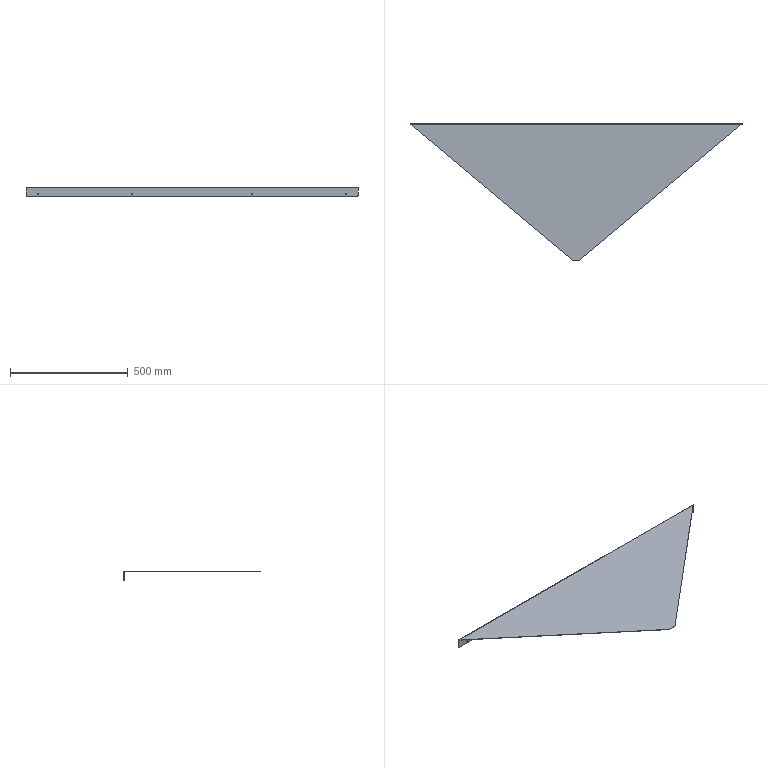Part | SolidWorks | features EdgeFlange 1, Fillet 1, FlatPattern 1, HoleWzd 1, SMBaseFlange 1, SheetMetal 1 | 1 solid | 24 faces | box 1412 x 580 x 40 mm | volume 567151 mm3 | cylinder 12 | plane 10 | spline 2 | commonest cylinder face diameters 4.5 x8 10 x2 0.2 x1 2.6 x1
STEP:
#1=CARTESIAN_POINT('',(50.,-1.2,-30.25));
#2=VERTEX_POINT('',#1);
#3=CARTESIAN_POINT('',(50.,-1.2,-25.75));
#4=VERTEX_POINT('',#3);
#5=CARTESIAN_POINT('',(50.,-1.2,-28.));
#6=DIRECTION('',(0.,1.,0.));
#7=DIRECTION('',(0.,0.,1.));
#8=AXIS2_PLACEMENT_3D('',#5,#6,#7);
#9=CIRCLE('',#8,2.25);
#10=EDGE_CURVE('',#2,#4,#9,.T.);
#11=ORIENTED_EDGE('',*,*,#10,.F.);
#12=CARTESIAN_POINT('',(50.,0.,-30.25));
#13=VERTEX_POINT('',#12);
#14=CARTESIAN_POINT('',(50.,0.,-30.25));
#15=DIRECTION('',(0.,1.,0.));
#16=VECTOR('',#15,1000.);
#17=LINE('',#14,#16);
#18=EDGE_CURVE('',#2,#13,#17,.T.);
#19=ORIENTED_EDGE('',*,*,#18,.T.);
#20=CARTESIAN_POINT('',(50.,0.,-25.75));
#21=VERTEX_POINT('',#20);
#22=CARTESIAN_POINT('',(50.,0.,-28.));
#23=DIRECTION('',(0.,1.,0.));
#24=DIRECTION('',(0.,0.,1.));
#25=AXIS2_PLACEMENT_3D('',#22,#23,#24);
#26=CIRCLE('',#25,2.25);
#27=EDGE_CURVE('',#13,#21,#26,.T.);
#28=ORIENTED_EDGE('',*,*,#27,.T.);
#29=CARTESIAN_POINT('',(50.,0.,-25.75));
#30=DIRECTION('',(0.,1.,0.));
#31=VECTOR('',#30,1000.);
#32=LINE('',#29,#31);
#33=EDGE_CURVE('',#4,#21,#32,.T.);
#34=ORIENTED_EDGE('',*,*,#33,.F.);
#35=EDGE_LOOP('',(#11,#19,#28,#34));
#36=FACE_OUTER_BOUND('',#35,.T.);
#37=CARTESIAN_POINT('',(50.,0.,-28.));
#38=DIRECTION('',(0.,1.,0.));
#39=DIRECTION('',(0.,0.,1.));
#40=AXIS2_PLACEMENT_3D('',#37,#38,#39);
#41=CYLINDRICAL_SURFACE('',#40,2.25);
#42=ADVANCED_FACE('',(#36),#41,.F.);
#43=CARTESIAN_POINT('',(1362.,-1.2,-30.25));
#44=VERTEX_POINT('',#43);
#45=CARTESIAN_POINT('',(1362.,-1.2,-25.75));
#46=VERTEX_POINT('',#45);
#47=CARTESIAN_POINT('',(1362.,-1.2,-28.));
#48=DIRECTION('',(0.,1.,0.));
#49=DIRECTION('',(0.,0.,1.));
#50=AXIS2_PLACEMENT_3D('',#47,#48,#49);
#51=CIRCLE('',#50,2.25);
#52=EDGE_CURVE('',#44,#46,#51,.T.);
#53=ORIENTED_EDGE('',*,*,#52,.F.);
#54=CARTESIAN_POINT('',(1362.,0.,-30.25));
#55=VERTEX_POINT('',#54);
#56=CARTESIAN_POINT('',(1362.,0.,-30.25));
#57=DIRECTION('',(0.,1.,0.));
#58=VECTOR('',#57,1000.);
#59=LINE('',#56,#58);
#60=EDGE_CURVE('',#44,#55,#59,.T.);
#61=ORIENTED_EDGE('',*,*,#60,.T.);
#62=CARTESIAN_POINT('',(1362.,0.,-25.75));
#63=VERTEX_POINT('',#62);
#64=CARTESIAN_POINT('',(1362.,0.,-28.));
#65=DIRECTION('',(0.,1.,0.));
#66=DIRECTION('',(0.,0.,1.));
#67=AXIS2_PLACEMENT_3D('',#64,#65,#66);
#68=CIRCLE('',#67,2.25);
#69=EDGE_CURVE('',#55,#63,#68,.T.);
#70=ORIENTED_EDGE('',*,*,#69,.T.);
#71=CARTESIAN_POINT('',(1362.,0.,-25.75));
#72=DIRECTION('',(0.,1.,0.));
#73=VECTOR('',#72,1000.);
#74=LINE('',#71,#73);
#75=EDGE_CURVE('',#46,#63,#74,.T.);
#76=ORIENTED_EDGE('',*,*,#75,.F.);
#77=EDGE_LOOP('',(#53,#61,#70,#76));
#78=FACE_OUTER_BOUND('',#77,.T.);
#79=CARTESIAN_POINT('',(1362.,0.,-28.));
#80=DIRECTION('',(0.,1.,0.));
#81=DIRECTION('',(0.,0.,1.));
#82=AXIS2_PLACEMENT_3D('',#79,#80,#81);
#83=CYLINDRICAL_SURFACE('',#82,2.25);
#84=ADVANCED_FACE('',(#78),#83,.F.);
#85=CARTESIAN_POINT('',(962.,-1.2,-30.25));
#86=VERTEX_POINT('',#85);
#87=CARTESIAN_POINT('',(962.,-1.2,-25.75));
#88=VERTEX_POINT('',#87);
#89=CARTESIAN_POINT('',(962.,-1.2,-28.));
#90=DIRECTION('',(0.,1.,0.));
#91=DIRECTION('',(0.,0.,1.));
#92=AXIS2_PLACEMENT_3D('',#89,#90,#91);
#93=CIRCLE('',#92,2.25);
#94=EDGE_CURVE('',#86,#88,#93,.T.);
#95=ORIENTED_EDGE('',*,*,#94,.F.);
#96=CARTESIAN_POINT('',(962.,0.,-30.25));
#97=VERTEX_POINT('',#96);
#98=CARTESIAN_POINT('',(962.,0.,-30.25));
#99=DIRECTION('',(0.,1.,0.));
#100=VECTOR('',#99,1000.);
#101=LINE('',#98,#100);
#102=EDGE_CURVE('',#86,#97,#101,.T.);
#103=ORIENTED_EDGE('',*,*,#102,.T.);
#104=CARTESIAN_POINT('',(962.,0.,-25.75));
#105=VERTEX_POINT('',#104);
#106=CARTESIAN_POINT('',(962.,0.,-28.));
#107=DIRECTION('',(0.,1.,0.));
#108=DIRECTION('',(0.,0.,1.));
#109=AXIS2_PLACEMENT_3D('',#106,#107,#108);
#110=CIRCLE('',#109,2.25);
#111=EDGE_CURVE('',#97,#105,#110,.T.);
#112=ORIENTED_EDGE('',*,*,#111,.T.);
#113=CARTESIAN_POINT('',(962.,0.,-25.75));
#114=DIRECTION('',(0.,1.,0.));
#115=VECTOR('',#114,1000.);
#116=LINE('',#113,#115);
#117=EDGE_CURVE('',#88,#105,#116,.T.);
#118=ORIENTED_EDGE('',*,*,#117,.F.);
#119=EDGE_LOOP('',(#95,#103,#112,#118));
#120=FACE_OUTER_BOUND('',#119,.T.);
#121=CARTESIAN_POINT('',(962.,0.,-28.));
#122=DIRECTION('',(0.,1.,0.));
#123=DIRECTION('',(0.,0.,1.));
#124=AXIS2_PLACEMENT_3D('',#121,#122,#123);
#125=CYLINDRICAL_SURFACE('',#124,2.25);
#126=ADVANCED_FACE('',(#120),#125,.F.);
#127=CARTESIAN_POINT('',(450.,-1.2,-30.25));
#128=VERTEX_POINT('',#127);
#129=CARTESIAN_POINT('',(450.,-1.2,-25.75));
#130=VERTEX_POINT('',#129);
#131=CARTESIAN_POINT('',(450.,-1.2,-28.));
#132=DIRECTION('',(0.,1.,0.));
#133=DIRECTION('',(0.,0.,1.));
#134=AXIS2_PLACEMENT_3D('',#131,#132,#133);
#135=CIRCLE('',#134,2.25);
#136=EDGE_CURVE('',#128,#130,#135,.T.);
#137=ORIENTED_EDGE('',*,*,#136,.F.);
#138=CARTESIAN_POINT('',(450.,0.,-30.25));
#139=VERTEX_POINT('',#138);
#140=CARTESIAN_POINT('',(450.,0.,-30.25));
#141=DIRECTION('',(0.,1.,0.));
#142=VECTOR('',#141,1000.);
#143=LINE('',#140,#142);
#144=EDGE_CURVE('',#128,#139,#143,.T.);
#145=ORIENTED_EDGE('',*,*,#144,.T.);
#146=CARTESIAN_POINT('',(450.,0.,-25.75));
#147=VERTEX_POINT('',#146);
#148=CARTESIAN_POINT('',(450.,0.,-28.));
#149=DIRECTION('',(0.,1.,0.));
#150=DIRECTION('',(0.,0.,1.));
#151=AXIS2_PLACEMENT_3D('',#148,#149,#150);
#152=CIRCLE('',#151,2.25);
#153=EDGE_CURVE('',#139,#147,#152,.T.);
#154=ORIENTED_EDGE('',*,*,#153,.T.);
#155=CARTESIAN_POINT('',(450.,0.,-25.75));
#156=DIRECTION('',(0.,1.,0.));
#157=VECTOR('',#156,1000.);
#158=LINE('',#155,#157);
#159=EDGE_CURVE('',#130,#147,#158,.T.);
#160=ORIENTED_EDGE('',*,*,#159,.F.);
#161=EDGE_LOOP('',(#137,#145,#154,#160));
#162=FACE_OUTER_BOUND('',#161,.T.);
#163=CARTESIAN_POINT('',(450.,0.,-28.));
#164=DIRECTION('',(0.,1.,0.));
#165=DIRECTION('',(0.,0.,1.));
#166=AXIS2_PLACEMENT_3D('',#163,#164,#165);
#167=CYLINDRICAL_SURFACE('',#166,2.25);
#168=ADVANCED_FACE('',(#162),#167,.F.);
#169=CARTESIAN_POINT('',(1.548,-1.3,0.));
#170=VERTEX_POINT('',#169);
#171=CARTESIAN_POINT('',(690.727,-580.,0.));
#172=VERTEX_POINT('',#171);
#173=CARTESIAN_POINT('',(690.727,-580.,0.));
#174=DIRECTION('',(0.7658,-0.6431,0.));
#175=VECTOR('',#174,1000.);
#176=LINE('',#173,#175);
#177=EDGE_CURVE('',#170,#172,#176,.T.);
#178=ORIENTED_EDGE('',*,*,#177,.F.);
#179=CARTESIAN_POINT('',(1.548,-1.3,-1.2));
#180=VERTEX_POINT('',#179);
#181=CARTESIAN_POINT('',(1.548,-1.3,-1.2));
#182=DIRECTION('',(0.,0.,1.));
#183=VECTOR('',#182,1000.);
#184=LINE('',#181,#183);
#185=EDGE_CURVE('',#180,#170,#184,.T.);
#186=ORIENTED_EDGE('',*,*,#185,.F.);
#187=CARTESIAN_POINT('',(690.727,-580.,-1.2));
#188=VERTEX_POINT('',#187);
#189=CARTESIAN_POINT('',(690.727,-580.,-1.2));
#190=DIRECTION('',(0.7658,-0.6431,0.));
#191=VECTOR('',#190,1000.);
#192=LINE('',#189,#191);
#193=EDGE_CURVE('',#180,#188,#192,.T.);
#194=ORIENTED_EDGE('',*,*,#193,.T.);
#195=CARTESIAN_POINT('',(690.727,-580.,-1.2));
#196=DIRECTION('',(0.,0.,1.));
#197=VECTOR('',#196,1000.);
#198=LINE('',#195,#197);
#199=EDGE_CURVE('',#188,#172,#198,.T.);
#200=ORIENTED_EDGE('',*,*,#199,.T.);
#201=EDGE_LOOP('',(#178,#186,#194,#200));
#202=FACE_OUTER_BOUND('',#201,.T.);
#203=CARTESIAN_POINT('',(690.727,-580.,-1.2));
#204=DIRECTION('',(-0.6431,-0.7658,0.));
#205=DIRECTION('',(0.7658,-0.6431,0.));
#206=AXIS2_PLACEMENT_3D('',#203,#204,#205);
#207=PLANE('',#206);
#208=ADVANCED_FACE('',(#202),#207,.T.);
#209=CARTESIAN_POINT('',(721.273,-580.,-1.2));
#210=VERTEX_POINT('',#209);
#211=CARTESIAN_POINT('',(1410.452,-1.3,-1.2));
#212=VERTEX_POINT('',#211);
#213=CARTESIAN_POINT('',(1412.,0.,-1.2));
#214=DIRECTION('',(0.7658,0.6431,0.));
#215=VECTOR('',#214,1000.);
#216=LINE('',#213,#215);
#217=EDGE_CURVE('',#210,#212,#216,.T.);
#218=ORIENTED_EDGE('',*,*,#217,.T.);
#219=CARTESIAN_POINT('',(1410.452,-1.3,0.));
#220=VERTEX_POINT('',#219);
#221=CARTESIAN_POINT('',(1410.452,-1.3,-1.2));
#222=DIRECTION('',(0.,0.,1.));
#223=VECTOR('',#222,1000.);
#224=LINE('',#221,#223);
#225=EDGE_CURVE('',#212,#220,#224,.T.);
#226=ORIENTED_EDGE('',*,*,#225,.T.);
#227=CARTESIAN_POINT('',(721.273,-580.,0.));
#228=VERTEX_POINT('',#227);
#229=CARTESIAN_POINT('',(1412.,0.,0.));
#230=DIRECTION('',(0.7658,0.6431,0.));
#231=VECTOR('',#230,1000.);
#232=LINE('',#229,#231);
#233=EDGE_CURVE('',#228,#220,#232,.T.);
#234=ORIENTED_EDGE('',*,*,#233,.F.);
#235=CARTESIAN_POINT('',(721.273,-580.,-1.2));
#236=DIRECTION('',(0.,0.,1.));
#237=VECTOR('',#236,1000.);
#238=LINE('',#235,#237);
#239=EDGE_CURVE('',#210,#228,#238,.T.);
#240=ORIENTED_EDGE('',*,*,#239,.F.);
#241=EDGE_LOOP('',(#218,#226,#234,#240));
#242=FACE_OUTER_BOUND('',#241,.T.);
#243=CARTESIAN_POINT('',(1412.,0.,-1.2));
#244=DIRECTION('',(0.6431,-0.7658,0.));
#245=DIRECTION('',(0.7658,0.6431,0.));
#246=AXIS2_PLACEMENT_3D('',#243,#244,#245);
#247=PLANE('',#246);
#248=ADVANCED_FACE('',(#242),#247,.T.);
#249=CARTESIAN_POINT('',(1412.,-1.3,-1.2));
#250=DIRECTION('',(-1.,0.,0.));
#251=VECTOR('',#250,1000.);
#252=LINE('',#249,#251);
#253=EDGE_CURVE('',#212,#180,#252,.T.);
#254=ORIENTED_EDGE('',*,*,#253,.F.);
#255=ORIENTED_EDGE('',*,*,#217,.F.);
#256=CARTESIAN_POINT('',(721.273,-580.,-1.2));
#257=DIRECTION('',(1.,0.,0.));
#258=VECTOR('',#257,1000.);
#259=LINE('',#256,#258);
#260=EDGE_CURVE('',#188,#210,#259,.T.);
#261=ORIENTED_EDGE('',*,*,#260,.F.);
#262=ORIENTED_EDGE('',*,*,#193,.F.);
#263=EDGE_LOOP('',(#254,#255,#261,#262));
#264=FACE_OUTER_BOUND('',#263,.T.);
#265=CARTESIAN_POINT('',(0.,0.,-1.2));
#266=DIRECTION('',(0.,0.,1.));
#267=DIRECTION('',(1.,0.,0.));
#268=AXIS2_PLACEMENT_3D('',#265,#266,#267);
#269=PLANE('',#268);
#270=ADVANCED_FACE('',(#264),#269,.F.);
#271=ORIENTED_EDGE('',*,*,#233,.T.);
#272=CARTESIAN_POINT('',(1412.,-1.3,0.));
#273=DIRECTION('',(-1.,0.,0.));
#274=VECTOR('',#273,1000.);
#275=LINE('',#272,#274);
#276=EDGE_CURVE('',#220,#170,#275,.T.);
#277=ORIENTED_EDGE('',*,*,#276,.T.);
#278=ORIENTED_EDGE('',*,*,#177,.T.);
#279=CARTESIAN_POINT('',(721.273,-580.,0.));
#280=DIRECTION('',(1.,0.,0.));
#281=VECTOR('',#280,1000.);
#282=LINE('',#279,#281);
#283=EDGE_CURVE('',#172,#228,#282,.T.);
#284=ORIENTED_EDGE('',*,*,#283,.T.);
#285=EDGE_LOOP('',(#271,#277,#278,#284));
#286=FACE_OUTER_BOUND('',#285,.T.);
#287=CARTESIAN_POINT('',(0.,0.,0.));
#288=DIRECTION('',(0.,0.,1.));
#289=DIRECTION('',(1.,0.,0.));
#290=AXIS2_PLACEMENT_3D('',#287,#288,#289);
#291=PLANE('',#290);
#292=ADVANCED_FACE('',(#286),#291,.T.);
#293=ORIENTED_EDGE('',*,*,#283,.F.);
#294=ORIENTED_EDGE('',*,*,#199,.F.);
#295=ORIENTED_EDGE('',*,*,#260,.T.);
#296=ORIENTED_EDGE('',*,*,#239,.T.);
#297=EDGE_LOOP('',(#293,#294,#295,#296));
#298=FACE_OUTER_BOUND('',#297,.T.);
#299=CARTESIAN_POINT('',(721.273,-580.,-1.2));
#300=DIRECTION('',(0.,-1.,0.));
#301=DIRECTION('',(0.,0.,-1.));
#302=AXIS2_PLACEMENT_3D('',#299,#300,#301);
#303=PLANE('',#302);
#304=ADVANCED_FACE('',(#298),#303,.T.);
#305=CARTESIAN_POINT('',(0.,-1.2,-1.3));
#306=VERTEX_POINT('',#305);
#307=CARTESIAN_POINT('',(0.,0.,-1.3));
#308=VERTEX_POINT('',#307);
#309=CARTESIAN_POINT('',(0.,0.,-1.3));
#310=DIRECTION('',(0.,1.,0.));
#311=VECTOR('',#310,1000.);
#312=LINE('',#309,#311);
#313=EDGE_CURVE('',#306,#308,#312,.T.);
#314=ORIENTED_EDGE('',*,*,#313,.F.);
#315=CARTESIAN_POINT('',(1.548,-1.3,-1.2));
#316=CARTESIAN_POINT('',(1.29,-1.274,-1.2));
#317=CARTESIAN_POINT('',(1.032,-1.248,-1.211));
#318=CARTESIAN_POINT('',(0.5161,-1.211,-1.248));
#319=CARTESIAN_POINT('',(0.258,-1.2,-1.274));
#320=CARTESIAN_POINT('',(0.,-1.2,-1.3));
#321=B_SPLINE_CURVE_WITH_KNOTS('',3,(#315,#316,#317,#318,#319,#320),.UNSPECIFIED.,.F.,.F.,(4,2,4),(0.,0.5,1.),.UNSPECIFIED.);
#322=EDGE_CURVE('',#180,#306,#321,.T.);
#323=ORIENTED_EDGE('',*,*,#322,.F.);
#324=ORIENTED_EDGE('',*,*,#185,.T.);
#325=CARTESIAN_POINT('',(1.548,-1.3,0.));
#326=CARTESIAN_POINT('',(1.418,-1.128,0.));
#327=CARTESIAN_POINT('',(1.291,-0.9602,-0.03358));
#328=CARTESIAN_POINT('',(1.031,-0.6438,-0.1648));
#329=CARTESIAN_POINT('',(0.9042,-0.5022,-0.2594));
#330=CARTESIAN_POINT('',(0.6445,-0.2599,-0.5015));
#331=CARTESIAN_POINT('',(0.5173,-0.1649,-0.6438));
#332=CARTESIAN_POINT('',(0.2586,-0.03398,-0.9589));
#333=CARTESIAN_POINT('',(0.1301,0.,-1.128));
#334=CARTESIAN_POINT('',(0.,0.,-1.3));
#335=B_SPLINE_CURVE_WITH_KNOTS('',3,(#325,#326,#327,#328,#329,#330,#331,#332,#333,#334),.UNSPECIFIED.,.F.,.F.,(4,2,2,2,4),(0.,0.0006388,0.001278,0.001916,0.002555),.UNSPECIFIED.);
#336=EDGE_CURVE('',#170,#308,#335,.T.);
#337=ORIENTED_EDGE('',*,*,#336,.T.);
#338=EDGE_LOOP('',(#314,#323,#324,#337));
#339=FACE_OUTER_BOUND('',#338,.T.);
#340=CARTESIAN_POINT('',(1.548,-1.3,0.012));
#341=CARTESIAN_POINT('',(1.419,-1.128,0.012));
#342=CARTESIAN_POINT('',(1.29,-0.9566,-0.02215));
#343=CARTESIAN_POINT('',(1.032,-0.6393,-0.1536));
#344=CARTESIAN_POINT('',(0.9031,-0.4937,-0.2508));
#345=CARTESIAN_POINT('',(0.6451,-0.2508,-0.4937));
#346=CARTESIAN_POINT('',(0.5161,-0.1536,-0.6393));
#347=CARTESIAN_POINT('',(0.258,-0.02215,-0.9566));
#348=CARTESIAN_POINT('',(0.129,0.012,-1.128));
#349=CARTESIAN_POINT('',(0.,0.012,-1.3));
#350=CARTESIAN_POINT('',(1.548,-1.3,0.));
#351=CARTESIAN_POINT('',(1.419,-1.13,0.));
#352=CARTESIAN_POINT('',(1.29,-0.9597,-0.03384));
#353=CARTESIAN_POINT('',(1.032,-0.6453,-0.1641));
#354=CARTESIAN_POINT('',(0.9031,-0.5011,-0.2604));
#355=CARTESIAN_POINT('',(0.6451,-0.2604,-0.5011));
#356=CARTESIAN_POINT('',(0.5161,-0.1641,-0.6453));
#357=CARTESIAN_POINT('',(0.258,-0.03384,-0.9597));
#358=CARTESIAN_POINT('',(0.129,0.,-1.13));
#359=CARTESIAN_POINT('',(0.,0.,-1.3));
#360=CARTESIAN_POINT('',(1.548,-1.3,-1.2));
#361=CARTESIAN_POINT('',(1.419,-1.287,-1.2));
#362=CARTESIAN_POINT('',(1.29,-1.274,-1.203));
#363=CARTESIAN_POINT('',(1.032,-1.25,-1.213));
#364=CARTESIAN_POINT('',(0.9031,-1.239,-1.22));
#365=CARTESIAN_POINT('',(0.6451,-1.22,-1.239));
#366=CARTESIAN_POINT('',(0.5161,-1.213,-1.25));
#367=CARTESIAN_POINT('',(0.258,-1.203,-1.274));
#368=CARTESIAN_POINT('',(0.129,-1.2,-1.287));
#369=CARTESIAN_POINT('',(0.,-1.2,-1.3));
#370=B_SPLINE_SURFACE_WITH_KNOTS('',1,3,((#340,#341,#342,#343,#344,#345,#346,#347,#348,#349),(#350,#351,#352,#353,#354,#355,#356,#357,#358,#359),(#360,#361,#362,#363,#364,#365,#366,#367,#368,#369)),.UNSPECIFIED.,.F.,.F.,.F.,(2,1,2),(4,2,2,2,4),(-0.01,0.,1.),(0.,0.25,0.5,0.75,1.),.UNSPECIFIED.);
#371=ADVANCED_FACE('',(#339),#370,.F.);
#372=CARTESIAN_POINT('',(1412.,-1.2,-1.3));
#373=VERTEX_POINT('',#372);
#374=CARTESIAN_POINT('',(1412.,-1.2,-1.3));
#375=CARTESIAN_POINT('',(1411.742,-1.2,-1.274));
#376=CARTESIAN_POINT('',(1411.484,-1.211,-1.248));
#377=CARTESIAN_POINT('',(1410.968,-1.248,-1.211));
#378=CARTESIAN_POINT('',(1410.71,-1.274,-1.2));
#379=CARTESIAN_POINT('',(1410.452,-1.3,-1.2));
#380=B_SPLINE_CURVE_WITH_KNOTS('',3,(#374,#375,#376,#377,#378,#379),.UNSPECIFIED.,.F.,.F.,(4,2,4),(0.,0.5,1.),.UNSPECIFIED.);
#381=EDGE_CURVE('',#373,#212,#380,.T.);
#382=ORIENTED_EDGE('',*,*,#381,.F.);
#383=CARTESIAN_POINT('',(1412.,0.,-1.3));
#384=VERTEX_POINT('',#383);
#385=CARTESIAN_POINT('',(1412.,-1.2,-1.3));
#386=DIRECTION('',(0.,1.,0.));
#387=VECTOR('',#386,1000.);
#388=LINE('',#385,#387);
#389=EDGE_CURVE('',#373,#384,#388,.T.);
#390=ORIENTED_EDGE('',*,*,#389,.T.);
#391=CARTESIAN_POINT('',(1412.,0.,-1.3));
#392=CARTESIAN_POINT('',(1411.87,0.,-1.128));
#393=CARTESIAN_POINT('',(1411.742,-0.03358,-0.9602));
#394=CARTESIAN_POINT('',(1411.483,-0.1648,-0.6438));
#395=CARTESIAN_POINT('',(1411.356,-0.2594,-0.5022));
#396=CARTESIAN_POINT('',(1411.096,-0.5015,-0.2599));
#397=CARTESIAN_POINT('',(1410.969,-0.6438,-0.1649));
#398=CARTESIAN_POINT('',(1410.71,-0.9589,-0.03398));
#399=CARTESIAN_POINT('',(1410.582,-1.128,0.));
#400=CARTESIAN_POINT('',(1410.452,-1.3,0.));
#401=B_SPLINE_CURVE_WITH_KNOTS('',3,(#391,#392,#393,#394,#395,#396,#397,#398,#399,#400),.UNSPECIFIED.,.F.,.F.,(4,2,2,2,4),(0.,0.0006388,0.001278,0.001916,0.002555),.UNSPECIFIED.);
#402=EDGE_CURVE('',#384,#220,#401,.T.);
#403=ORIENTED_EDGE('',*,*,#402,.T.);
#404=ORIENTED_EDGE('',*,*,#225,.F.);
#405=EDGE_LOOP('',(#382,#390,#403,#404));
#406=FACE_OUTER_BOUND('',#405,.T.);
#407=CARTESIAN_POINT('',(1412.,0.012,-1.3));
#408=CARTESIAN_POINT('',(1411.871,0.012,-1.128));
#409=CARTESIAN_POINT('',(1411.742,-0.02215,-0.9566));
#410=CARTESIAN_POINT('',(1411.484,-0.1536,-0.6393));
#411=CARTESIAN_POINT('',(1411.355,-0.2508,-0.4937));
#412=CARTESIAN_POINT('',(1411.097,-0.4937,-0.2508));
#413=CARTESIAN_POINT('',(1410.968,-0.6393,-0.1536));
#414=CARTESIAN_POINT('',(1410.71,-0.9566,-0.02215));
#415=CARTESIAN_POINT('',(1410.581,-1.128,0.012));
#416=CARTESIAN_POINT('',(1410.452,-1.3,0.012));
#417=CARTESIAN_POINT('',(1412.,0.,-1.3));
#418=CARTESIAN_POINT('',(1411.871,0.,-1.13));
#419=CARTESIAN_POINT('',(1411.742,-0.03384,-0.9597));
#420=CARTESIAN_POINT('',(1411.484,-0.1641,-0.6453));
#421=CARTESIAN_POINT('',(1411.355,-0.2604,-0.5011));
#422=CARTESIAN_POINT('',(1411.097,-0.5011,-0.2604));
#423=CARTESIAN_POINT('',(1410.968,-0.6453,-0.1641));
#424=CARTESIAN_POINT('',(1410.71,-0.9597,-0.03384));
#425=CARTESIAN_POINT('',(1410.581,-1.13,0.));
#426=CARTESIAN_POINT('',(1410.452,-1.3,0.));
#427=CARTESIAN_POINT('',(1412.,-1.2,-1.3));
#428=CARTESIAN_POINT('',(1411.871,-1.2,-1.287));
#429=CARTESIAN_POINT('',(1411.742,-1.203,-1.274));
#430=CARTESIAN_POINT('',(1411.484,-1.213,-1.25));
#431=CARTESIAN_POINT('',(1411.355,-1.22,-1.239));
#432=CARTESIAN_POINT('',(1411.097,-1.239,-1.22));
#433=CARTESIAN_POINT('',(1410.968,-1.25,-1.213));
#434=CARTESIAN_POINT('',(1410.71,-1.274,-1.203));
#435=CARTESIAN_POINT('',(1410.581,-1.287,-1.2));
#436=CARTESIAN_POINT('',(1410.452,-1.3,-1.2));
#437=B_SPLINE_SURFACE_WITH_KNOTS('',1,3,((#407,#408,#409,#410,#411,#412,#413,#414,#415,#416),(#417,#418,#419,#420,#421,#422,#423,#424,#425,#426),(#427,#428,#429,#430,#431,#432,#433,#434,#435,#436)),.UNSPECIFIED.,.F.,.F.,.F.,(2,1,2),(4,2,2,2,4),(-0.01,0.,1.),(0.,0.25,0.5,0.75,1.),.UNSPECIFIED.);
#438=ADVANCED_FACE('',(#406),#437,.F.);
#439=ORIENTED_EDGE('',*,*,#276,.F.);
#440=ORIENTED_EDGE('',*,*,#402,.F.);
#441=CARTESIAN_POINT('',(0.,0.,-1.3));
#442=DIRECTION('',(1.,0.,0.));
#443=VECTOR('',#442,1000.);
#444=LINE('',#441,#443);
#445=EDGE_CURVE('',#308,#384,#444,.T.);
#446=ORIENTED_EDGE('',*,*,#445,.F.);
#447=ORIENTED_EDGE('',*,*,#336,.F.);
#448=EDGE_LOOP('',(#439,#440,#446,#447));
#449=FACE_OUTER_BOUND('',#448,.T.);
#450=CARTESIAN_POINT('',(1412.,-1.3,-1.3));
#451=DIRECTION('',(1.,0.,0.));
#452=DIRECTION('',(0.,1.,0.));
#453=AXIS2_PLACEMENT_3D('',#450,#451,#452);
#454=CYLINDRICAL_SURFACE('',#453,1.3);
#455=ADVANCED_FACE('',(#449),#454,.T.);
#456=ORIENTED_EDGE('',*,*,#253,.T.);
#457=ORIENTED_EDGE('',*,*,#322,.T.);
#458=CARTESIAN_POINT('',(0.,-1.2,-1.3));
#459=DIRECTION('',(1.,0.,0.));
#460=VECTOR('',#459,1000.);
#461=LINE('',#458,#460);
#462=EDGE_CURVE('',#306,#373,#461,.T.);
#463=ORIENTED_EDGE('',*,*,#462,.T.);
#464=ORIENTED_EDGE('',*,*,#381,.T.);
#465=EDGE_LOOP('',(#456,#457,#463,#464));
#466=FACE_OUTER_BOUND('',#465,.T.);
#467=CARTESIAN_POINT('',(1412.,-1.3,-1.3));
#468=DIRECTION('',(1.,0.,0.));
#469=DIRECTION('',(0.,1.,0.));
#470=AXIS2_PLACEMENT_3D('',#467,#468,#469);
#471=CYLINDRICAL_SURFACE('',#470,0.1);
#472=ADVANCED_FACE('',(#466),#471,.F.);
#473=CARTESIAN_POINT('',(1412.,-1.2,-35.));
#474=VERTEX_POINT('',#473);
#475=CARTESIAN_POINT('',(1412.,-1.2,0.));
#476=DIRECTION('',(0.,0.,1.));
#477=VECTOR('',#476,1000.);
#478=LINE('',#475,#477);
#479=EDGE_CURVE('',#474,#373,#478,.T.);
#480=ORIENTED_EDGE('',*,*,#479,.F.);
#481=CARTESIAN_POINT('',(1412.,0.,-35.));
#482=VERTEX_POINT('',#481);
#483=CARTESIAN_POINT('',(1412.,0.,-35.));
#484=DIRECTION('',(0.,1.,0.));
#485=VECTOR('',#484,1000.);
#486=LINE('',#483,#485);
#487=EDGE_CURVE('',#474,#482,#486,.T.);
#488=ORIENTED_EDGE('',*,*,#487,.T.);
#489=CARTESIAN_POINT('',(1412.,0.,-1.2));
#490=DIRECTION('',(0.,0.,1.));
#491=VECTOR('',#490,1000.);
#492=LINE('',#489,#491);
#493=EDGE_CURVE('',#482,#384,#492,.T.);
#494=ORIENTED_EDGE('',*,*,#493,.T.);
#495=ORIENTED_EDGE('',*,*,#389,.F.);
#496=EDGE_LOOP('',(#480,#488,#494,#495));
#497=FACE_OUTER_BOUND('',#496,.T.);
#498=CARTESIAN_POINT('',(1412.,0.,-1.2));
#499=DIRECTION('',(1.,0.,0.));
#500=DIRECTION('',(0.,1.,0.));
#501=AXIS2_PLACEMENT_3D('',#498,#499,#500);
#502=PLANE('',#501);
#503=ADVANCED_FACE('',(#497),#502,.T.);
#504=CARTESIAN_POINT('',(0.,0.,-35.));
#505=VERTEX_POINT('',#504);
#506=CARTESIAN_POINT('',(0.,0.,-40.));
#507=DIRECTION('',(0.,0.,-1.));
#508=VECTOR('',#507,1000.);
#509=LINE('',#506,#508);
#510=EDGE_CURVE('',#308,#505,#509,.T.);
#511=ORIENTED_EDGE('',*,*,#510,.T.);
#512=CARTESIAN_POINT('',(0.,-1.2,-35.));
#513=VERTEX_POINT('',#512);
#514=CARTESIAN_POINT('',(0.,0.,-35.));
#515=DIRECTION('',(0.,-1.,0.));
#516=VECTOR('',#515,1000.);
#517=LINE('',#514,#516);
#518=EDGE_CURVE('',#505,#513,#517,.T.);
#519=ORIENTED_EDGE('',*,*,#518,.T.);
#520=CARTESIAN_POINT('',(0.,-1.2,0.));
#521=DIRECTION('',(0.,0.,-1.));
#522=VECTOR('',#521,1000.);
#523=LINE('',#520,#522);
#524=EDGE_CURVE('',#306,#513,#523,.T.);
#525=ORIENTED_EDGE('',*,*,#524,.F.);
#526=ORIENTED_EDGE('',*,*,#313,.T.);
#527=EDGE_LOOP('',(#511,#519,#525,#526));
#528=FACE_OUTER_BOUND('',#527,.T.);
#529=CARTESIAN_POINT('',(0.,0.,-40.));
#530=DIRECTION('',(-1.,0.,0.));
#531=DIRECTION('',(0.,-1.,0.));
#532=AXIS2_PLACEMENT_3D('',#529,#530,#531);
#533=PLANE('',#532);
#534=ADVANCED_FACE('',(#528),#533,.T.);
#535=CARTESIAN_POINT('',(50.,0.,-28.));
#536=DIRECTION('',(0.,1.,0.));
#537=DIRECTION('',(0.,0.,1.));
#538=AXIS2_PLACEMENT_3D('',#535,#536,#537);
#539=CIRCLE('',#538,2.25);
#540=EDGE_CURVE('',#21,#13,#539,.T.);
#541=ORIENTED_EDGE('',*,*,#540,.F.);
#542=ORIENTED_EDGE('',*,*,#27,.F.);
#543=EDGE_LOOP('',(#541,#542));
#544=FACE_BOUND('',#543,.T.);
#545=CARTESIAN_POINT('',(1362.,0.,-28.));
#546=DIRECTION('',(0.,1.,0.));
#547=DIRECTION('',(0.,0.,1.));
#548=AXIS2_PLACEMENT_3D('',#545,#546,#547);
#549=CIRCLE('',#548,2.25);
#550=EDGE_CURVE('',#63,#55,#549,.T.);
#551=ORIENTED_EDGE('',*,*,#550,.F.);
#552=ORIENTED_EDGE('',*,*,#69,.F.);
#553=EDGE_LOOP('',(#551,#552));
#554=FACE_BOUND('',#553,.T.);
#555=CARTESIAN_POINT('',(962.,0.,-28.));
#556=DIRECTION('',(0.,1.,0.));
#557=DIRECTION('',(0.,0.,1.));
#558=AXIS2_PLACEMENT_3D('',#555,#556,#557);
#559=CIRCLE('',#558,2.25);
#560=EDGE_CURVE('',#105,#97,#559,.T.);
#561=ORIENTED_EDGE('',*,*,#560,.F.);
#562=ORIENTED_EDGE('',*,*,#111,.F.);
#563=EDGE_LOOP('',(#561,#562));
#564=FACE_BOUND('',#563,.T.);
#565=CARTESIAN_POINT('',(450.,0.,-28.));
#566=DIRECTION('',(0.,1.,0.));
#567=DIRECTION('',(0.,0.,1.));
#568=AXIS2_PLACEMENT_3D('',#565,#566,#567);
#569=CIRCLE('',#568,2.25);
#570=EDGE_CURVE('',#147,#139,#569,.T.);
#571=ORIENTED_EDGE('',*,*,#570,.F.);
#572=ORIENTED_EDGE('',*,*,#153,.F.);
#573=EDGE_LOOP('',(#571,#572));
#574=FACE_BOUND('',#573,.T.);
#575=CARTESIAN_POINT('',(5.,0.,-40.));
#576=VERTEX_POINT('',#575);
#577=CARTESIAN_POINT('',(1407.,0.,-40.));
#578=VERTEX_POINT('',#577);
#579=CARTESIAN_POINT('',(1412.,0.,-40.));
#580=DIRECTION('',(1.,0.,0.));
#581=VECTOR('',#580,1000.);
#582=LINE('',#579,#581);
#583=EDGE_CURVE('',#576,#578,#582,.T.);
#584=ORIENTED_EDGE('',*,*,#583,.F.);
#585=CARTESIAN_POINT('',(5.,0.,-35.));
#586=DIRECTION('',(0.,1.,0.));
#587=DIRECTION('',(0.,0.,1.));
#588=AXIS2_PLACEMENT_3D('',#585,#586,#587);
#589=CIRCLE('',#588,5.);
#590=EDGE_CURVE('',#576,#505,#589,.T.);
#591=ORIENTED_EDGE('',*,*,#590,.T.);
#592=ORIENTED_EDGE('',*,*,#510,.F.);
#593=ORIENTED_EDGE('',*,*,#445,.T.);
#594=ORIENTED_EDGE('',*,*,#493,.F.);
#595=CARTESIAN_POINT('',(1407.,0.,-35.));
#596=DIRECTION('',(0.,1.,0.));
#597=DIRECTION('',(0.,0.,1.));
#598=AXIS2_PLACEMENT_3D('',#595,#596,#597);
#599=CIRCLE('',#598,5.);
#600=EDGE_CURVE('',#482,#578,#599,.T.);
#601=ORIENTED_EDGE('',*,*,#600,.T.);
#602=EDGE_LOOP('',(#584,#591,#592,#593,#594,#601));
#603=FACE_OUTER_BOUND('',#602,.T.);
#604=CARTESIAN_POINT('',(0.,0.,0.));
#605=DIRECTION('',(0.,1.,0.));
#606=DIRECTION('',(0.,0.,1.));
#607=AXIS2_PLACEMENT_3D('',#604,#605,#606);
#608=PLANE('',#607);
#609=ADVANCED_FACE('',(#544,#554,#564,#574,#603),#608,.T.);
#610=CARTESIAN_POINT('',(50.,-1.2,-28.));
#611=DIRECTION('',(0.,1.,0.));
#612=DIRECTION('',(0.,0.,1.));
#613=AXIS2_PLACEMENT_3D('',#610,#611,#612);
#614=CIRCLE('',#613,2.25);
#615=EDGE_CURVE('',#4,#2,#614,.T.);
#616=ORIENTED_EDGE('',*,*,#615,.T.);
#617=ORIENTED_EDGE('',*,*,#10,.T.);
#618=EDGE_LOOP('',(#616,#617));
#619=FACE_BOUND('',#618,.T.);
#620=CARTESIAN_POINT('',(1362.,-1.2,-28.));
#621=DIRECTION('',(0.,1.,0.));
#622=DIRECTION('',(0.,0.,1.));
#623=AXIS2_PLACEMENT_3D('',#620,#621,#622);
#624=CIRCLE('',#623,2.25);
#625=EDGE_CURVE('',#46,#44,#624,.T.);
#626=ORIENTED_EDGE('',*,*,#625,.T.);
#627=ORIENTED_EDGE('',*,*,#52,.T.);
#628=EDGE_LOOP('',(#626,#627));
#629=FACE_BOUND('',#628,.T.);
#630=CARTESIAN_POINT('',(962.,-1.2,-28.));
#631=DIRECTION('',(0.,1.,0.));
#632=DIRECTION('',(0.,0.,1.));
#633=AXIS2_PLACEMENT_3D('',#630,#631,#632);
#634=CIRCLE('',#633,2.25);
#635=EDGE_CURVE('',#88,#86,#634,.T.);
#636=ORIENTED_EDGE('',*,*,#635,.T.);
#637=ORIENTED_EDGE('',*,*,#94,.T.);
#638=EDGE_LOOP('',(#636,#637));
#639=FACE_BOUND('',#638,.T.);
#640=CARTESIAN_POINT('',(450.,-1.2,-28.));
#641=DIRECTION('',(0.,1.,0.));
#642=DIRECTION('',(0.,0.,1.));
#643=AXIS2_PLACEMENT_3D('',#640,#641,#642);
#644=CIRCLE('',#643,2.25);
#645=EDGE_CURVE('',#130,#128,#644,.T.);
#646=ORIENTED_EDGE('',*,*,#645,.T.);
#647=ORIENTED_EDGE('',*,*,#136,.T.);
#648=EDGE_LOOP('',(#646,#647));
#649=FACE_BOUND('',#648,.T.);
#650=ORIENTED_EDGE('',*,*,#524,.T.);
#651=CARTESIAN_POINT('',(5.,-1.2,-40.));
#652=VERTEX_POINT('',#651);
#653=CARTESIAN_POINT('',(5.,-1.2,-35.));
#654=DIRECTION('',(0.,-1.,0.));
#655=DIRECTION('',(0.,0.,1.));
#656=AXIS2_PLACEMENT_3D('',#653,#654,#655);
#657=CIRCLE('',#656,5.);
#658=EDGE_CURVE('',#513,#652,#657,.T.);
#659=ORIENTED_EDGE('',*,*,#658,.T.);
#660=CARTESIAN_POINT('',(1407.,-1.2,-40.));
#661=VERTEX_POINT('',#660);
#662=CARTESIAN_POINT('',(0.,-1.2,-40.));
#663=DIRECTION('',(1.,0.,0.));
#664=VECTOR('',#663,1000.);
#665=LINE('',#662,#664);
#666=EDGE_CURVE('',#652,#661,#665,.T.);
#667=ORIENTED_EDGE('',*,*,#666,.T.);
#668=CARTESIAN_POINT('',(1407.,-1.2,-35.));
#669=DIRECTION('',(0.,-1.,0.));
#670=DIRECTION('',(0.,0.,1.));
#671=AXIS2_PLACEMENT_3D('',#668,#669,#670);
#672=CIRCLE('',#671,5.);
#673=EDGE_CURVE('',#661,#474,#672,.T.);
#674=ORIENTED_EDGE('',*,*,#673,.T.);
#675=ORIENTED_EDGE('',*,*,#479,.T.);
#676=ORIENTED_EDGE('',*,*,#462,.F.);
#677=EDGE_LOOP('',(#650,#659,#667,#674,#675,#676));
#678=FACE_OUTER_BOUND('',#677,.T.);
#679=CARTESIAN_POINT('',(0.,-1.2,0.));
#680=DIRECTION('',(0.,1.,0.));
#681=DIRECTION('',(0.,0.,1.));
#682=AXIS2_PLACEMENT_3D('',#679,#680,#681);
#683=PLANE('',#682);
#684=ADVANCED_FACE('',(#619,#629,#639,#649,#678),#683,.F.);
#685=ORIENTED_EDGE('',*,*,#666,.F.);
#686=CARTESIAN_POINT('',(5.,0.,-40.));
#687=DIRECTION('',(0.,1.,0.));
#688=VECTOR('',#687,1000.);
#689=LINE('',#686,#688);
#690=EDGE_CURVE('',#652,#576,#689,.T.);
#691=ORIENTED_EDGE('',*,*,#690,.T.);
#692=ORIENTED_EDGE('',*,*,#583,.T.);
#693=CARTESIAN_POINT('',(1407.,0.,-40.));
#694=DIRECTION('',(0.,-1.,0.));
#695=VECTOR('',#694,1000.);
#696=LINE('',#693,#695);
#697=EDGE_CURVE('',#578,#661,#696,.T.);
#698=ORIENTED_EDGE('',*,*,#697,.T.);
#699=EDGE_LOOP('',(#685,#691,#692,#698));
#700=FACE_OUTER_BOUND('',#699,.T.);
#701=CARTESIAN_POINT('',(1412.,0.,-40.));
#702=DIRECTION('',(0.,0.,-1.));
#703=DIRECTION('',(0.,1.,0.));
#704=AXIS2_PLACEMENT_3D('',#701,#702,#703);
#705=PLANE('',#704);
#706=ADVANCED_FACE('',(#700),#705,.T.);
#707=ORIENTED_EDGE('',*,*,#590,.F.);
#708=ORIENTED_EDGE('',*,*,#690,.F.);
#709=ORIENTED_EDGE('',*,*,#658,.F.);
#710=ORIENTED_EDGE('',*,*,#518,.F.);
#711=EDGE_LOOP('',(#707,#708,#709,#710));
#712=FACE_OUTER_BOUND('',#711,.T.);
#713=CARTESIAN_POINT('',(5.,0.,-35.));
#714=DIRECTION('',(0.,-1.,0.));
#715=DIRECTION('',(0.,0.,-1.));
#716=AXIS2_PLACEMENT_3D('',#713,#714,#715);
#717=CYLINDRICAL_SURFACE('',#716,5.);
#718=ADVANCED_FACE('',(#712),#717,.T.);
#719=ORIENTED_EDGE('',*,*,#600,.F.);
#720=ORIENTED_EDGE('',*,*,#487,.F.);
#721=ORIENTED_EDGE('',*,*,#673,.F.);
#722=ORIENTED_EDGE('',*,*,#697,.F.);
#723=EDGE_LOOP('',(#719,#720,#721,#722));
#724=FACE_OUTER_BOUND('',#723,.T.);
#725=CARTESIAN_POINT('',(1407.,0.,-35.));
#726=DIRECTION('',(0.,-1.,0.));
#727=DIRECTION('',(0.,0.,-1.));
#728=AXIS2_PLACEMENT_3D('',#725,#726,#727);
#729=CYLINDRICAL_SURFACE('',#728,5.);
#730=ADVANCED_FACE('',(#724),#729,.T.);
#731=ORIENTED_EDGE('',*,*,#144,.F.);
#732=ORIENTED_EDGE('',*,*,#645,.F.);
#733=ORIENTED_EDGE('',*,*,#159,.T.);
#734=ORIENTED_EDGE('',*,*,#570,.T.);
#735=EDGE_LOOP('',(#731,#732,#733,#734));
#736=FACE_OUTER_BOUND('',#735,.T.);
#737=CARTESIAN_POINT('',(450.,0.,-28.));
#738=DIRECTION('',(0.,1.,0.));
#739=DIRECTION('',(0.,0.,1.));
#740=AXIS2_PLACEMENT_3D('',#737,#738,#739);
#741=CYLINDRICAL_SURFACE('',#740,2.25);
#742=ADVANCED_FACE('',(#736),#741,.F.);
#743=ORIENTED_EDGE('',*,*,#102,.F.);
#744=ORIENTED_EDGE('',*,*,#635,.F.);
#745=ORIENTED_EDGE('',*,*,#117,.T.);
#746=ORIENTED_EDGE('',*,*,#560,.T.);
#747=EDGE_LOOP('',(#743,#744,#745,#746));
#748=FACE_OUTER_BOUND('',#747,.T.);
#749=CARTESIAN_POINT('',(962.,0.,-28.));
#750=DIRECTION('',(0.,1.,0.));
#751=DIRECTION('',(0.,0.,1.));
#752=AXIS2_PLACEMENT_3D('',#749,#750,#751);
#753=CYLINDRICAL_SURFACE('',#752,2.25);
#754=ADVANCED_FACE('',(#748),#753,.F.);
#755=ORIENTED_EDGE('',*,*,#60,.F.);
#756=ORIENTED_EDGE('',*,*,#625,.F.);
#757=ORIENTED_EDGE('',*,*,#75,.T.);
#758=ORIENTED_EDGE('',*,*,#550,.T.);
#759=EDGE_LOOP('',(#755,#756,#757,#758));
#760=FACE_OUTER_BOUND('',#759,.T.);
#761=CARTESIAN_POINT('',(1362.,0.,-28.));
#762=DIRECTION('',(0.,1.,0.));
#763=DIRECTION('',(0.,0.,1.));
#764=AXIS2_PLACEMENT_3D('',#761,#762,#763);
#765=CYLINDRICAL_SURFACE('',#764,2.25);
#766=ADVANCED_FACE('',(#760),#765,.F.);
#767=ORIENTED_EDGE('',*,*,#18,.F.);
#768=ORIENTED_EDGE('',*,*,#615,.F.);
#769=ORIENTED_EDGE('',*,*,#33,.T.);
#770=ORIENTED_EDGE('',*,*,#540,.T.);
#771=EDGE_LOOP('',(#767,#768,#769,#770));
#772=FACE_OUTER_BOUND('',#771,.T.);
#773=CARTESIAN_POINT('',(50.,0.,-28.));
#774=DIRECTION('',(0.,1.,0.));
#775=DIRECTION('',(0.,0.,1.));
#776=AXIS2_PLACEMENT_3D('',#773,#774,#775);
#777=CYLINDRICAL_SURFACE('',#776,2.25);
#778=ADVANCED_FACE('',(#772),#777,.F.);
#779=CLOSED_SHELL('',(#42,#84,#126,#168,#208,#248,#270,#292,#304,#371,#438,#455,#472,#503,#534,#609,#684,#706,#718,#730,#742,#754,#766,#778));
#780=MANIFOLD_SOLID_BREP('',#779);
#781=CARTESIAN_POINT('',(0.,0.,0.));
#782=DIRECTION('',(0.,0.,1.));
#783=DIRECTION('',(1.,0.,0.));
#784=AXIS2_PLACEMENT_3D('',#781,#782,#783);
#785=(LENGTH_UNIT()NAMED_UNIT(*)SI_UNIT(.MILLI.,.METRE.));
#786=UNCERTAINTY_MEASURE_WITH_UNIT(LENGTH_MEASURE(0.00001),#785,'','');
#787=(NAMED_UNIT(*)PLANE_ANGLE_UNIT()SI_UNIT($,.RADIAN.));
#788=(NAMED_UNIT(*)SI_UNIT($,.STERADIAN.)SOLID_ANGLE_UNIT());
#789=(GEOMETRIC_REPRESENTATION_CONTEXT(3)GLOBAL_UNCERTAINTY_ASSIGNED_CONTEXT((#786))GLOBAL_UNIT_ASSIGNED_CONTEXT((#785,#787,#788))REPRESENTATION_CONTEXT('',''));
#790=ADVANCED_BREP_SHAPE_REPRESENTATION('',(#780,#784),#789);